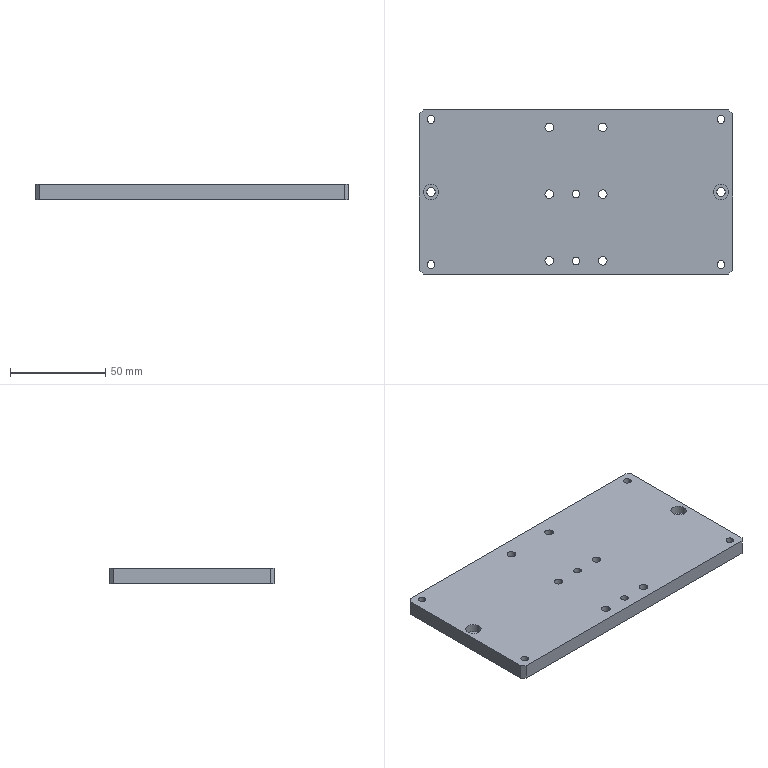Part | STEP file | QA-FB09 | 1 solid | 62 faces | box 164 x 86 x 8 mm | volume 109937 mm3 | cylinder 44 | plane 18 | commonest cylinder face diameters 4.5 x16 8 x16 4 x12